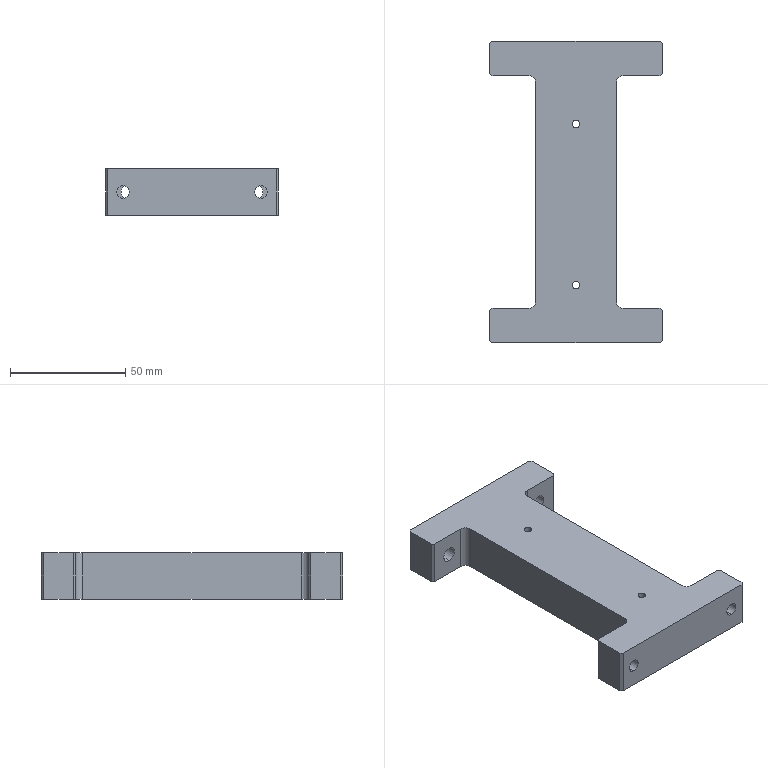Part | STEP file | 1 solid | 38 faces | box 75 x 131 x 20 mm | volume 113693 mm3 | plane 22 | cylinder 16 | commonest cylinder face diameters 3.3 x4 5.5 x4 6 x4 6.6 x4